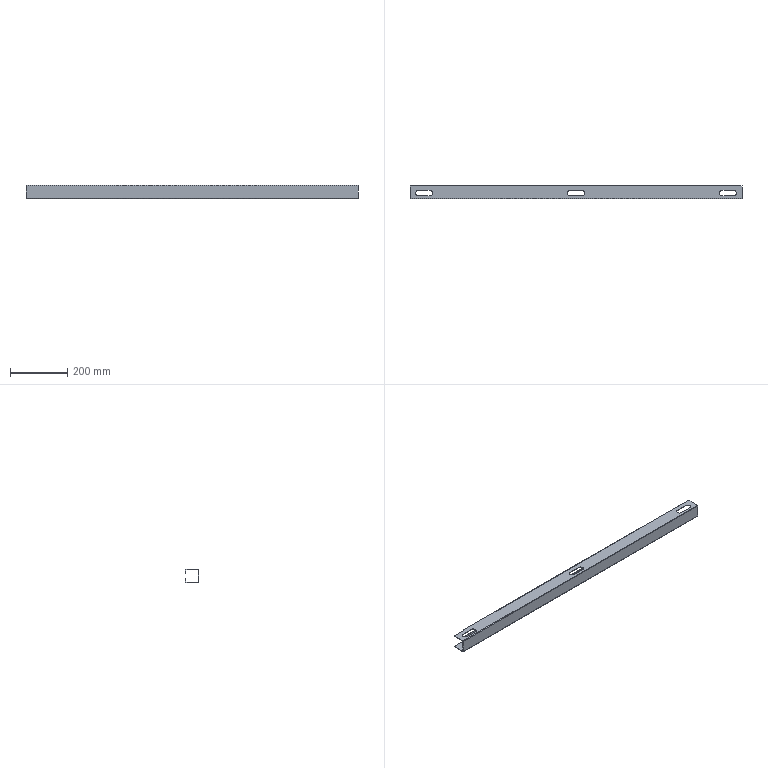Part | 1 solid | 70 faces | box 1159 x 48 x 46 mm | volume 270900 mm3 | plane 50 | cylinder 20 | commonest cylinder face diameters 20 x12 0.4 x4 3.4 x4